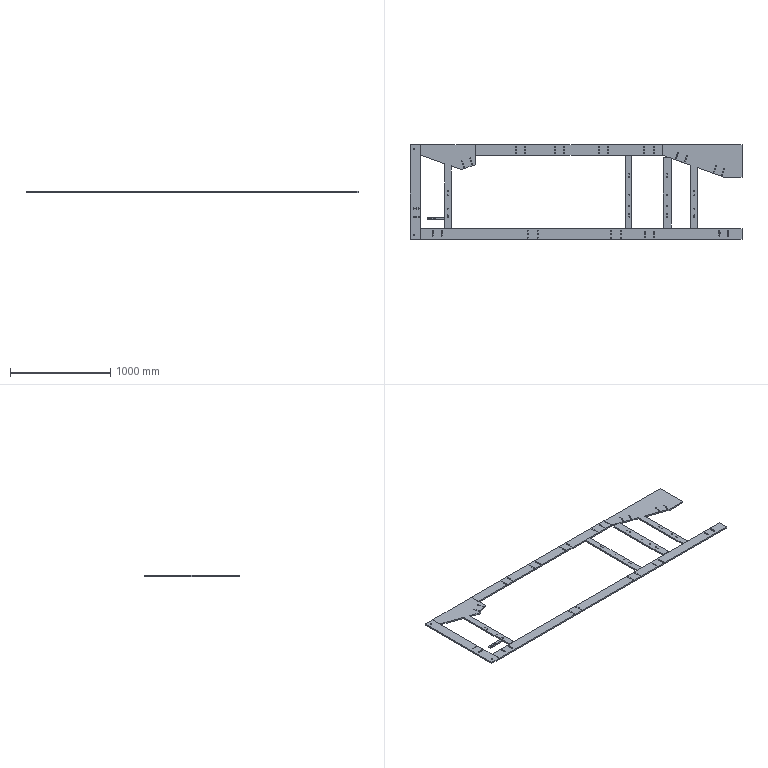Part | STEP file | 40A-00290-01-05 | 7 solids | 270 faces | box 3316 x 940 x 14 mm | volume 15103628 mm3 | cylinder 212 | plane 58 | commonest cylinder face diameters 10.2 x104 12 x52 10 x16 8.5 x14 8.8 x14 6.8 x4